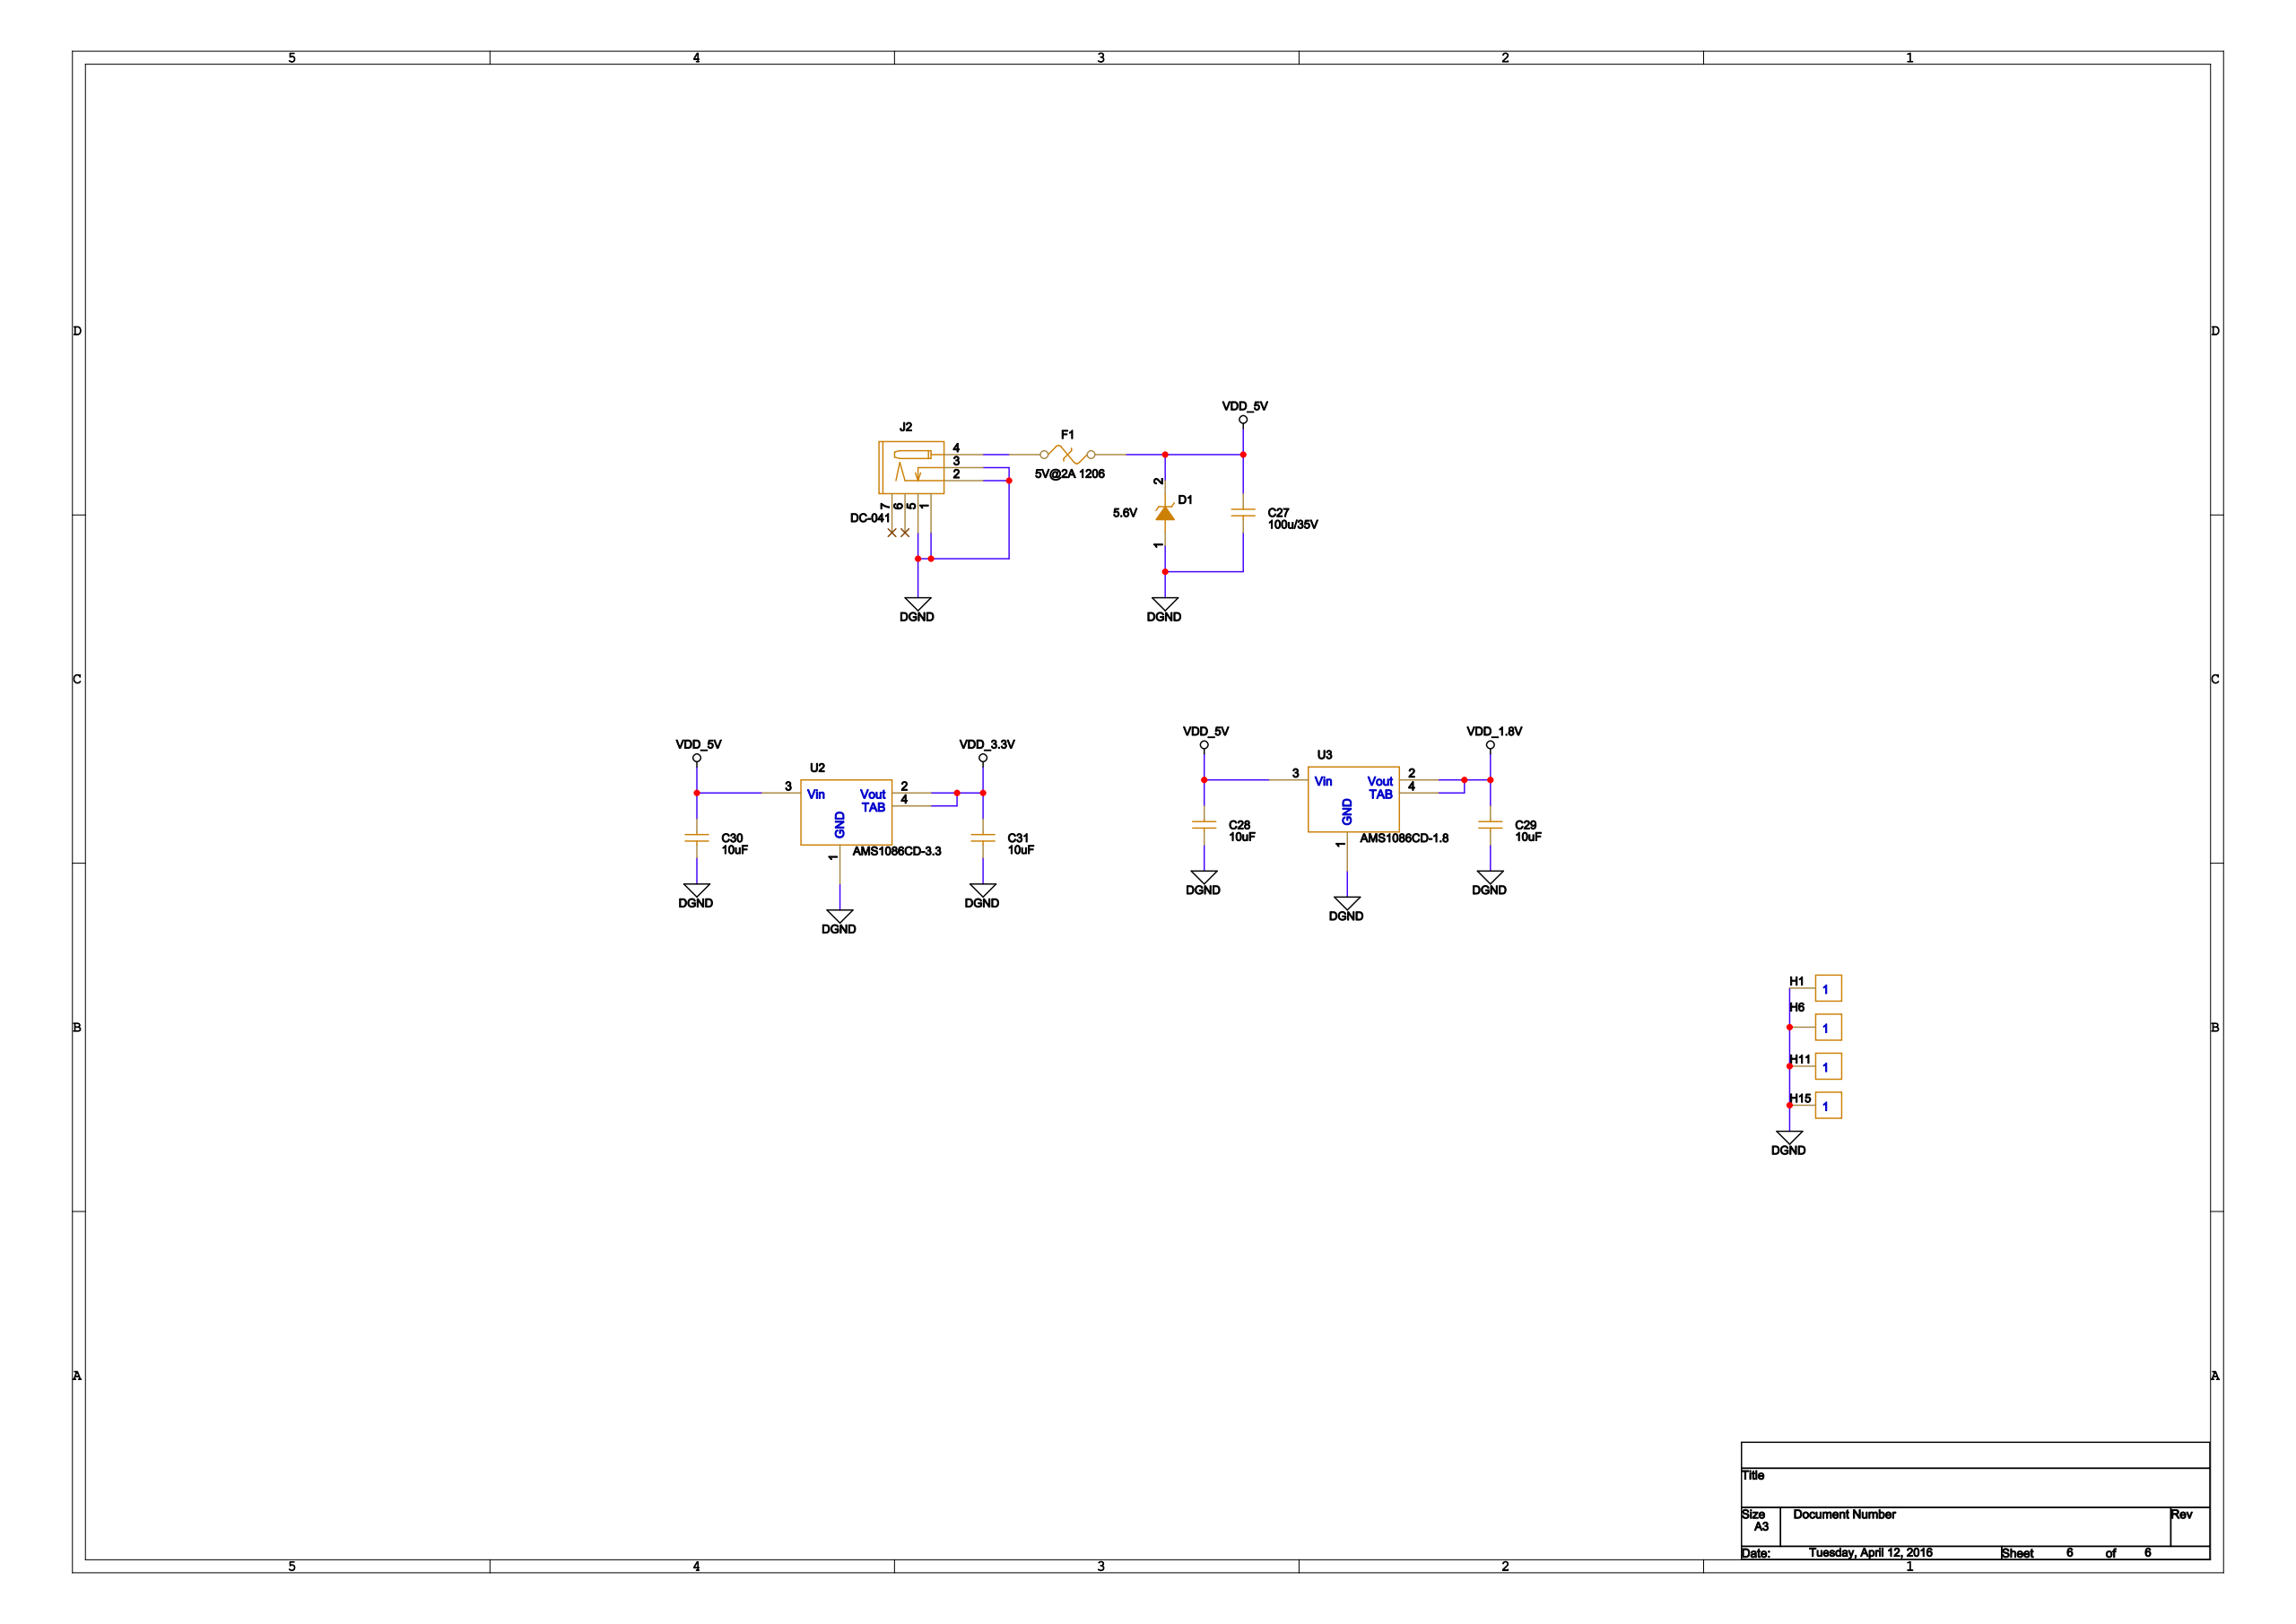Circuit board | Cadence Allegro | 85 parts | 48 nets | one sheet of the schematic
Parts on this sheet (reference | value | footprint):
C27 | 100u/35V | SMD6
C28 | 10uF | C0805
C29 | 10uF | C0805
C30 | 10uF | C0805
C31 | 10uF | C0805
D1 | 5.6V | DO-214AA-SMB
F1 | 5V@2A 1206 | F2410
H1 | CON1 | MH_125_
H6 | CON1 | MH_125_
H11 | CON1 | MH_125_
H15 | CON1 | MH_125_
J2 | DC-041 | DC-041
U2 | AMS1086CD-3.3 | TO-252
U3 | AMS1086CD-1.8 | TO-252
Nets of these parts (net: part-pin ...):
VDD_5V: C27-1 C28-1 C30-1 D1-2 F1-2 U2-3 U3-3
DGND: C27-2 C28-2 C29-2 C30-2 C31-2 D1-1 H1-1 H6-1 H11-1 H15-1 J2-1 J2-2 J2-3 J2-5 U2-1 U3-1
VDD_1.8V: C29-1 U3-2 U3-4
VDD_3.3V: C31-1 U2-2 U2-4
N9806730: F1-1 J2-4